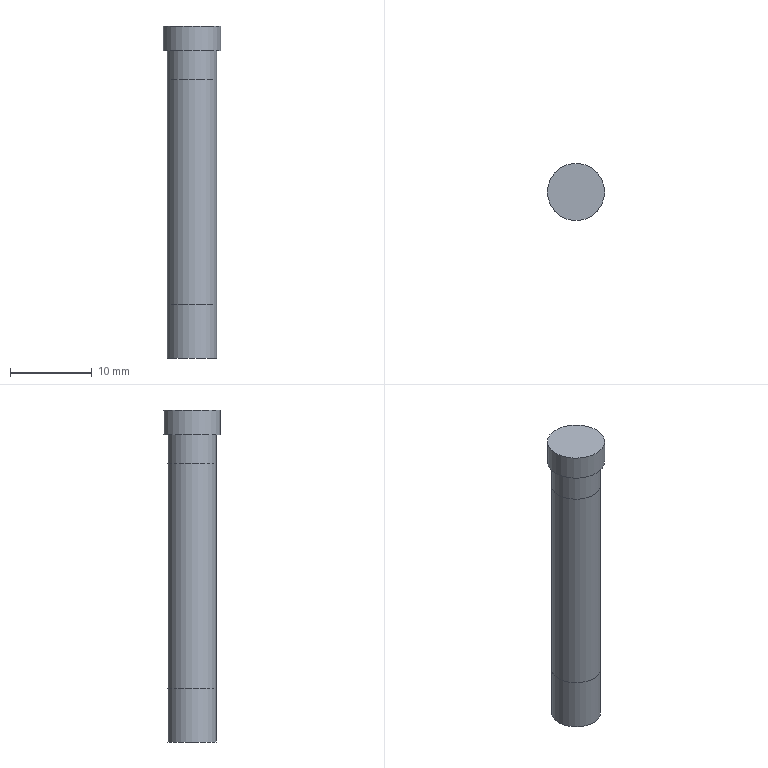Part | NX | features BREP 2 | 2 solids | 10 faces | box 7 x 7 x 40.6 mm | volume 2018 mm3 | plane 5 | cylinder 3 | torus 1 | cone 1 | commonest cylinder face diameters 6 x1 6.008 x1 7 x1
STEP:
#1=CARTESIAN_POINT('',(3.5,0.,-3.));
#2=VERTEX_POINT('',#1);
#3=CARTESIAN_POINT('',(0.,0.,-3.));
#4=DIRECTION('',(0.,0.,1.));
#5=DIRECTION('',(1.,0.,0.));
#6=AXIS2_PLACEMENT_3D('',#3,#4,#5);
#7=CIRCLE('',#6,3.5);
#8=EDGE_CURVE('',#2,#2,#7,.T.);
#9=ORIENTED_EDGE('',*,*,#8,.T.);
#10=EDGE_LOOP('',(#9));
#11=FACE_BOUND('',#10,.T.);
#12=CARTESIAN_POINT('',(3.5,0.,0.));
#13=VERTEX_POINT('',#12);
#14=CARTESIAN_POINT('',(0.,0.,0.));
#15=DIRECTION('',(0.,0.,1.));
#16=DIRECTION('',(1.,0.,0.));
#17=AXIS2_PLACEMENT_3D('',#14,#15,#16);
#18=CIRCLE('',#17,3.5);
#19=EDGE_CURVE('',#13,#13,#18,.T.);
#20=ORIENTED_EDGE('',*,*,#19,.F.);
#21=EDGE_LOOP('',(#20));
#22=FACE_BOUND('',#21,.T.);
#23=CARTESIAN_POINT('',(0.,0.,-3.));
#24=DIRECTION('',(0.,0.,1.));
#25=DIRECTION('',(-1.,0.,0.));
#26=AXIS2_PLACEMENT_3D('',#23,#24,#25);
#27=CYLINDRICAL_SURFACE('',#26,3.5);
#28=ADVANCED_FACE('',(#11,#22),#27,.T.);
#29=CARTESIAN_POINT('',(-3.,0.,-3.));
#30=VERTEX_POINT('',#29);
#31=CARTESIAN_POINT('',(0.,0.,-3.));
#32=DIRECTION('',(0.,0.,-1.));
#33=DIRECTION('',(-1.,0.,0.));
#34=AXIS2_PLACEMENT_3D('',#31,#32,#33);
#35=CIRCLE('',#34,3.);
#36=EDGE_CURVE('',#30,#30,#35,.T.);
#37=ORIENTED_EDGE('',*,*,#36,.F.);
#38=EDGE_LOOP('',(#37));
#39=FACE_BOUND('',#38,.T.);
#40=ORIENTED_EDGE('',*,*,#8,.F.);
#41=EDGE_LOOP('',(#40));
#42=FACE_BOUND('',#41,.T.);
#43=CARTESIAN_POINT('',(0.,0.,-3.));
#44=DIRECTION('',(0.,0.,1.));
#45=DIRECTION('',(-1.,0.,0.));
#46=AXIS2_PLACEMENT_3D('',#43,#44,#45);
#47=PLANE('',#46);
#48=ADVANCED_FACE('',(#39,#42),#47,.F.);
#49=ORIENTED_EDGE('',*,*,#19,.T.);
#50=EDGE_LOOP('',(#49));
#51=FACE_BOUND('',#50,.T.);
#52=CARTESIAN_POINT('',(0.,0.,0.));
#53=DIRECTION('',(0.,0.,1.));
#54=DIRECTION('',(-1.,0.,0.));
#55=AXIS2_PLACEMENT_3D('',#52,#53,#54);
#56=PLANE('',#55);
#57=ADVANCED_FACE('',(#51),#56,.T.);
#58=ORIENTED_EDGE('',*,*,#36,.T.);
#59=EDGE_LOOP('',(#58));
#60=FACE_BOUND('',#59,.T.);
#61=CARTESIAN_POINT('',(-3.,0.,-40.6));
#62=VERTEX_POINT('',#61);
#63=CARTESIAN_POINT('',(0.,0.,-40.6));
#64=DIRECTION('',(0.,0.,-1.));
#65=DIRECTION('',(-1.,0.,0.));
#66=AXIS2_PLACEMENT_3D('',#63,#64,#65);
#67=CIRCLE('',#66,3.);
#68=EDGE_CURVE('',#62,#62,#67,.T.);
#69=ORIENTED_EDGE('',*,*,#68,.F.);
#70=EDGE_LOOP('',(#69));
#71=FACE_BOUND('',#70,.T.);
#72=CARTESIAN_POINT('',(0.,0.,-3.));
#73=DIRECTION('',(0.,0.,-1.));
#74=DIRECTION('',(1.,0.,0.));
#75=AXIS2_PLACEMENT_3D('',#72,#73,#74);
#76=CYLINDRICAL_SURFACE('',#75,3.);
#77=ADVANCED_FACE('',(#60,#71),#76,.T.);
#78=ORIENTED_EDGE('',*,*,#68,.T.);
#79=EDGE_LOOP('',(#78));
#80=FACE_BOUND('',#79,.T.);
#81=CARTESIAN_POINT('',(0.,0.,-40.6));
#82=DIRECTION('',(0.,0.,-1.));
#83=DIRECTION('',(1.,0.,0.));
#84=AXIS2_PLACEMENT_3D('',#81,#82,#83);
#85=PLANE('',#84);
#86=ADVANCED_FACE('',(#80),#85,.T.);
#87=CLOSED_SHELL('',(#28,#48,#57,#77,#86));
#88=MANIFOLD_SOLID_BREP('',#87);
#89=CARTESIAN_POINT('',(3.004,0.,-34.));
#90=VERTEX_POINT('',#89);
#91=CARTESIAN_POINT('',(0.,0.,-34.));
#92=DIRECTION('',(0.,0.,1.));
#93=DIRECTION('',(1.,0.,0.));
#94=AXIS2_PLACEMENT_3D('',#91,#92,#93);
#95=CIRCLE('',#94,3.004);
#96=EDGE_CURVE('',#90,#90,#95,.T.);
#97=ORIENTED_EDGE('',*,*,#96,.T.);
#98=EDGE_LOOP('',(#97));
#99=FACE_BOUND('',#98,.T.);
#100=CARTESIAN_POINT('',(3.004,0.,-6.5));
#101=VERTEX_POINT('',#100);
#102=CARTESIAN_POINT('',(0.,0.,-6.5));
#103=DIRECTION('',(0.,0.,-1.));
#104=DIRECTION('',(1.,0.,0.));
#105=AXIS2_PLACEMENT_3D('',#102,#103,#104);
#106=CIRCLE('',#105,3.004);
#107=EDGE_CURVE('',#101,#101,#106,.T.);
#108=ORIENTED_EDGE('',*,*,#107,.T.);
#109=EDGE_LOOP('',(#108));
#110=FACE_BOUND('',#109,.T.);
#111=CARTESIAN_POINT('',(0.,0.,-35.));
#112=DIRECTION('',(0.,0.,1.));
#113=DIRECTION('',(-1.,0.,0.));
#114=AXIS2_PLACEMENT_3D('',#111,#112,#113);
#115=CYLINDRICAL_SURFACE('',#114,3.004);
#116=ADVANCED_FACE('',(#99,#110),#115,.T.);
#117=CARTESIAN_POINT('',(2.736,0.,-35.));
#118=VERTEX_POINT('',#117);
#119=CARTESIAN_POINT('',(0.,0.,-35.));
#120=DIRECTION('',(0.,0.,-1.));
#121=DIRECTION('',(1.,0.,0.));
#122=AXIS2_PLACEMENT_3D('',#119,#120,#121);
#123=CIRCLE('',#122,2.736);
#124=EDGE_CURVE('',#118,#118,#123,.T.);
#125=ORIENTED_EDGE('',*,*,#124,.T.);
#126=EDGE_LOOP('',(#125));
#127=FACE_BOUND('',#126,.T.);
#128=CARTESIAN_POINT('',(0.,0.,-35.));
#129=DIRECTION('',(0.,0.,1.));
#130=DIRECTION('',(-1.,0.,0.));
#131=AXIS2_PLACEMENT_3D('',#128,#129,#130);
#132=PLANE('',#131);
#133=ADVANCED_FACE('',(#127),#132,.F.);
#134=CARTESIAN_POINT('',(1.504,0.,-5.));
#135=VERTEX_POINT('',#134);
#136=CARTESIAN_POINT('',(0.,0.,-5.));
#137=DIRECTION('',(0.,0.,1.));
#138=DIRECTION('',(1.,0.,0.));
#139=AXIS2_PLACEMENT_3D('',#136,#137,#138);
#140=CIRCLE('',#139,1.504);
#141=EDGE_CURVE('',#135,#135,#140,.T.);
#142=ORIENTED_EDGE('',*,*,#141,.T.);
#143=EDGE_LOOP('',(#142));
#144=FACE_BOUND('',#143,.T.);
#145=CARTESIAN_POINT('',(0.,0.,-5.));
#146=DIRECTION('',(0.,0.,1.));
#147=DIRECTION('',(-1.,0.,0.));
#148=AXIS2_PLACEMENT_3D('',#145,#146,#147);
#149=PLANE('',#148);
#150=ADVANCED_FACE('',(#144),#149,.T.);
#151=ORIENTED_EDGE('',*,*,#107,.F.);
#152=EDGE_LOOP('',(#151));
#153=FACE_BOUND('',#152,.T.);
#154=ORIENTED_EDGE('',*,*,#141,.F.);
#155=EDGE_LOOP('',(#154));
#156=FACE_BOUND('',#155,.T.);
#157=CARTESIAN_POINT('',(0.,0.,-6.5));
#158=DIRECTION('',(0.,0.,1.));
#159=DIRECTION('',(-1.,0.,0.));
#160=AXIS2_PLACEMENT_3D('',#157,#158,#159);
#161=TOROIDAL_SURFACE('',#160,1.504,1.5);
#162=ADVANCED_FACE('',(#153,#156),#161,.T.);
#163=ORIENTED_EDGE('',*,*,#124,.F.);
#164=EDGE_LOOP('',(#163));
#165=FACE_BOUND('',#164,.T.);
#166=ORIENTED_EDGE('',*,*,#96,.F.);
#167=EDGE_LOOP('',(#166));
#168=FACE_BOUND('',#167,.T.);
#169=CARTESIAN_POINT('',(0.,0.,-34.));
#170=DIRECTION('',(0.,0.,1.));
#171=DIRECTION('',(-1.,0.,0.));
#172=AXIS2_PLACEMENT_3D('',#169,#170,#171);
#173=CONICAL_SURFACE('',#172,3.004,0.2618);
#174=ADVANCED_FACE('',(#165,#168),#173,.T.);
#175=CLOSED_SHELL('',(#116,#133,#150,#162,#174));
#176=MANIFOLD_SOLID_BREP('',#175);
#177=(LENGTH_UNIT()NAMED_UNIT(*)SI_UNIT(.MILLI.,.METRE.));
#178=UNCERTAINTY_MEASURE_WITH_UNIT(LENGTH_MEASURE(0.00001),#177,'','');
#179=(NAMED_UNIT(*)PLANE_ANGLE_UNIT()SI_UNIT($,.RADIAN.));
#180=(NAMED_UNIT(*)SI_UNIT($,.STERADIAN.)SOLID_ANGLE_UNIT());
#181=(GEOMETRIC_REPRESENTATION_CONTEXT(3)GLOBAL_UNCERTAINTY_ASSIGNED_CONTEXT((#178))GLOBAL_UNIT_ASSIGNED_CONTEXT((#177,#179,#180))REPRESENTATION_CONTEXT('',''));
#182=ADVANCED_BREP_SHAPE_REPRESENTATION('',(#88,#176),#181);